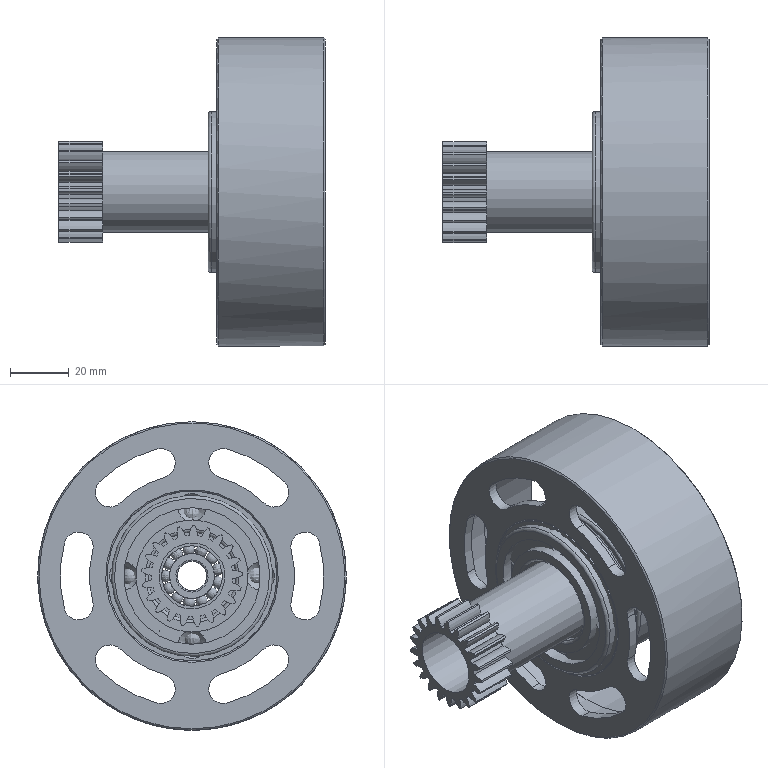Part | NX | features BREP 5 | 7 solids | 419 faces | box 91 x 105.4 x 105.4 mm | volume 127711 mm3 | cylinder 156 | torus 150 | sphere 66 | plane 32 | cone 15 | commonest cylinder face diameters 12.6 x42 27.748 x21 34.55 x21 10 x14 70 x6 90 x6